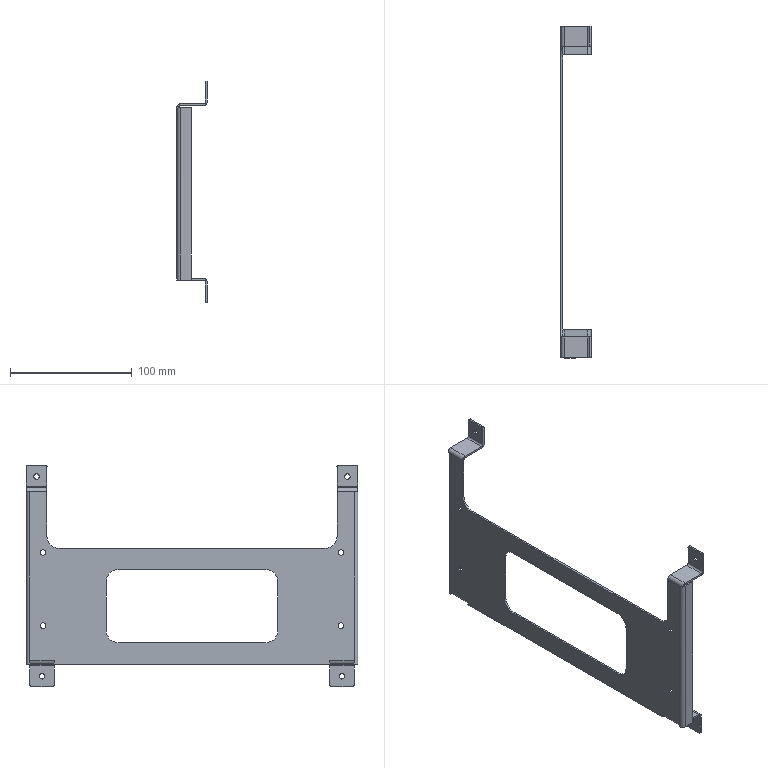Part | NX | features BREP 1 | 1 solid | 102 faces | box 24.9 x 272 x 181.457 mm | volume 37056 mm3 | plane 52 | cylinder 50 | commonest cylinder face diameters 3 x18 4.5 x16 6 x10 20 x6